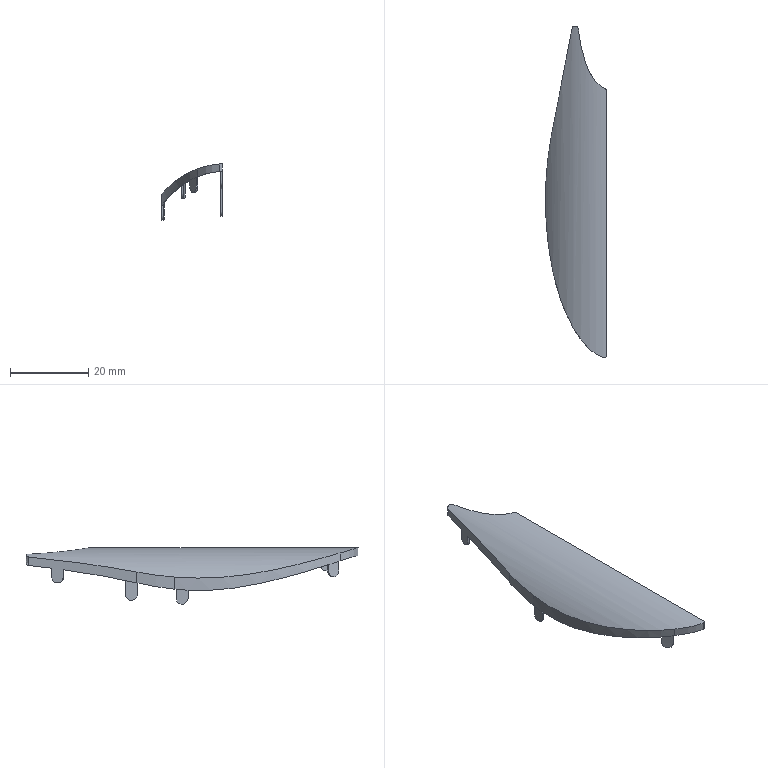Part | STEP file | 1 solid | 50 faces | box 15.6 x 84.944 x 14.464 mm | volume 720.197 mm3 | cylinder 20 | plane 16 | spline 14 | commonest cylinder face diameters 3 x8 40.2 x6 0.2 x1 1.2 x1 43.02 x1 44 x1